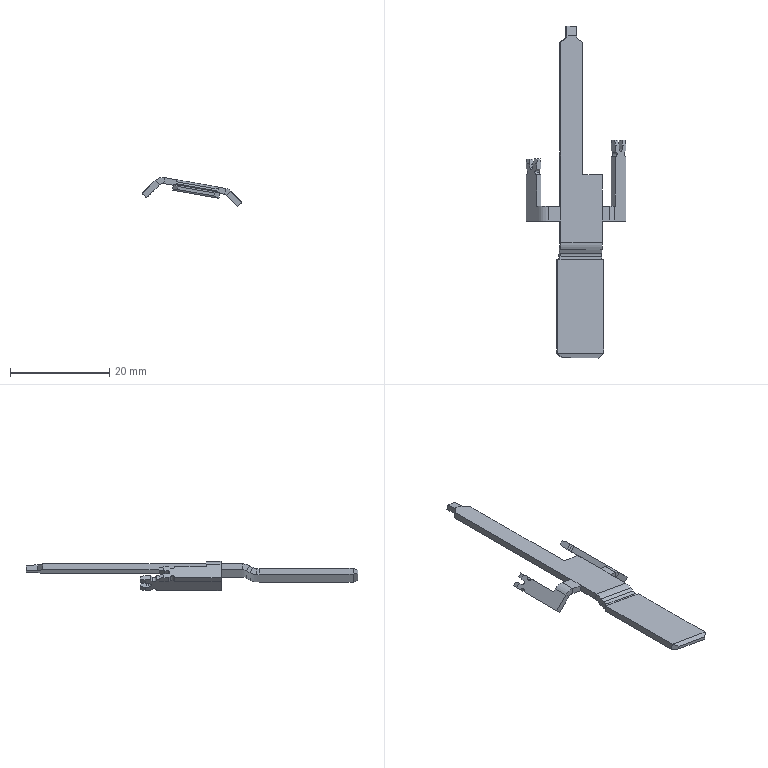Part | SolidWorks | features BaseBody 1 | 1 solid | 105 faces | box 20.099 x 66.9 x 5.857 mm | volume 673.523 mm3 | plane 89 | cylinder 16 | commonest cylinder face diameters 1 x7 0.8 x1 1.28 x1 2 x1 3 x1 3.6 x1